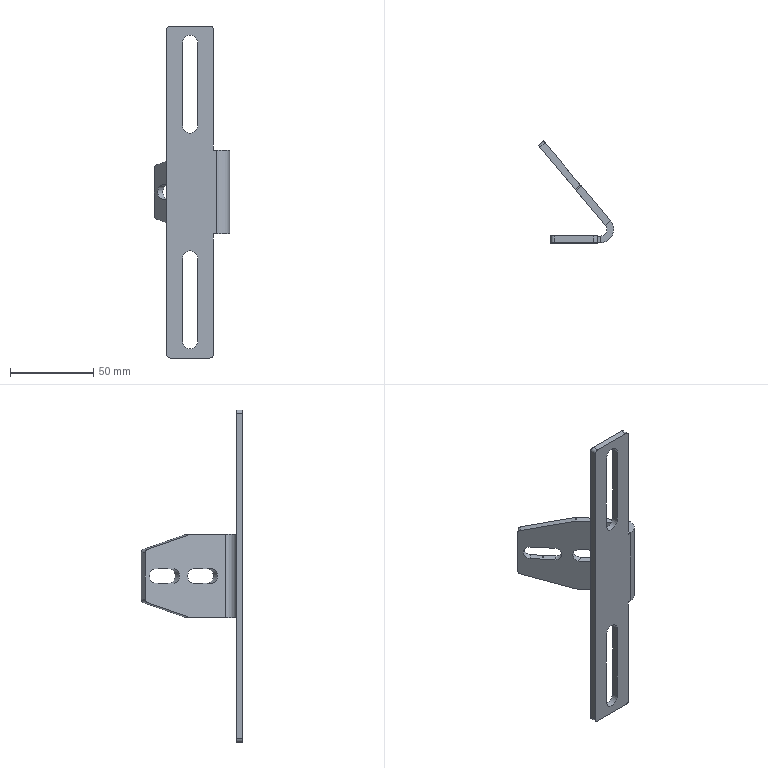Part | STEP file | Bracket for support | 1 solid | 56 faces | box 45.331 x 61.284 x 200 mm | volume 31041 mm3 | plane 32 | cylinder 24 | commonest cylinder face diameters 4 x10 8.49 x4 8.5 x4 9.2 x4 8 x1 16 x1